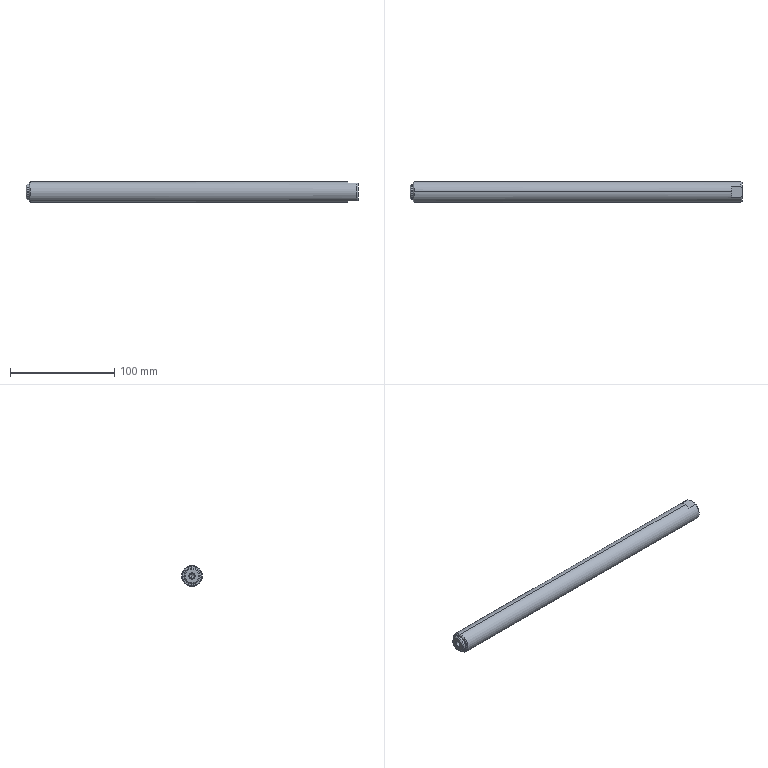Part | STEP file | sfpg20_315_f3_p15_m6_sc305_2_03 | 1 solid | 25 faces | box 318 x 20 x 20 mm | volume 98846 mm3 | cone 10 | plane 7 | cylinder 6 | spline 2 | commonest cylinder face diameters 4.917 x2 15 x2 20 x2